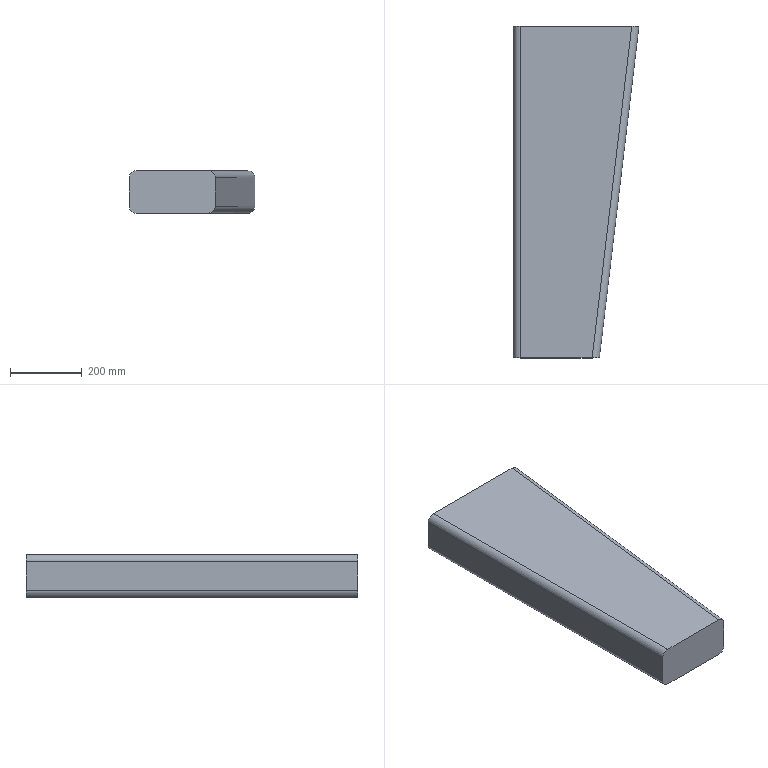Part | SolidWorks | features Extrusion 1, Fillet 1 | 1 solid | 10 faces | box 350 x 923 x 118 mm | volume 31811585 mm3 | plane 6 | cylinder 4 | commonest cylinder face diameters 40 x4
STEP:
#1=CARTESIAN_POINT('',(0.,923.,98.));
#2=VERTEX_POINT('',#1);
#3=CARTESIAN_POINT('',(0.,923.,20.));
#4=VERTEX_POINT('',#3);
#5=CARTESIAN_POINT('',(0.,923.,118.));
#6=DIRECTION('',(0.,0.,-1.));
#7=VECTOR('',#6,1000.);
#8=LINE('',#5,#7);
#9=EDGE_CURVE('',#2,#4,#8,.T.);
#10=ORIENTED_EDGE('',*,*,#9,.T.);
#11=CARTESIAN_POINT('',(0.,0.,20.));
#12=VERTEX_POINT('',#11);
#13=CARTESIAN_POINT('',(0.,923.,20.));
#14=DIRECTION('',(0.,-1.,0.));
#15=VECTOR('',#14,1000.);
#16=LINE('',#13,#15);
#17=EDGE_CURVE('',#4,#12,#16,.T.);
#18=ORIENTED_EDGE('',*,*,#17,.T.);
#19=CARTESIAN_POINT('',(0.,0.,98.));
#20=VERTEX_POINT('',#19);
#21=CARTESIAN_POINT('',(0.,0.,118.));
#22=DIRECTION('',(0.,0.,-1.));
#23=VECTOR('',#22,1000.);
#24=LINE('',#21,#23);
#25=EDGE_CURVE('',#20,#12,#24,.T.);
#26=ORIENTED_EDGE('',*,*,#25,.F.);
#27=CARTESIAN_POINT('',(0.,923.,98.));
#28=DIRECTION('',(0.,1.,0.));
#29=VECTOR('',#28,1000.);
#30=LINE('',#27,#29);
#31=EDGE_CURVE('',#20,#2,#30,.T.);
#32=ORIENTED_EDGE('',*,*,#31,.T.);
#33=EDGE_LOOP('',(#10,#18,#26,#32));
#34=FACE_OUTER_BOUND('',#33,.T.);
#35=CARTESIAN_POINT('',(0.,923.,118.));
#36=DIRECTION('',(1.,0.,0.));
#37=DIRECTION('',(0.,0.,-1.));
#38=AXIS2_PLACEMENT_3D('',#35,#36,#37);
#39=PLANE('',#38);
#40=ADVANCED_FACE('',(#34),#39,.F.);
#41=ORIENTED_EDGE('',*,*,#25,.T.);
#42=CARTESIAN_POINT('',(20.,0.,0.));
#43=VERTEX_POINT('',#42);
#44=CARTESIAN_POINT('',(20.,0.,20.));
#45=DIRECTION('',(0.,-1.,0.));
#46=DIRECTION('',(0.,0.,1.));
#47=AXIS2_PLACEMENT_3D('',#44,#45,#46);
#48=CIRCLE('',#47,20.);
#49=EDGE_CURVE('',#12,#43,#48,.T.);
#50=ORIENTED_EDGE('',*,*,#49,.T.);
#51=CARTESIAN_POINT('',(219.858,0.,0.));
#52=VERTEX_POINT('',#51);
#53=CARTESIAN_POINT('',(0.,0.,0.));
#54=DIRECTION('',(1.,0.,0.));
#55=VECTOR('',#54,1000.);
#56=LINE('',#53,#55);
#57=EDGE_CURVE('',#43,#52,#56,.T.);
#58=ORIENTED_EDGE('',*,*,#57,.T.);
#59=CARTESIAN_POINT('',(240.,0.,20.));
#60=VERTEX_POINT('',#59);
#61=CARTESIAN_POINT('',(219.858,0.,0.));
#62=CARTESIAN_POINT('',(231.657,0.,0.));
#63=CARTESIAN_POINT('',(240.,0.,8.284));
#64=CARTESIAN_POINT('',(240.,0.,20.));
#65=(BOUNDED_CURVE()B_SPLINE_CURVE(3,(#61,#62,#63,#64),.UNSPECIFIED.,.F.,.F.)B_SPLINE_CURVE_WITH_KNOTS((4,4),(4.712,6.283),.UNSPECIFIED.)CURVE()GEOMETRIC_REPRESENTATION_ITEM()RATIONAL_B_SPLINE_CURVE((1.,0.8047,0.8047,1.))REPRESENTATION_ITEM(''));
#66=EDGE_CURVE('',#52,#60,#65,.T.);
#67=ORIENTED_EDGE('',*,*,#66,.T.);
#68=CARTESIAN_POINT('',(240.,0.,98.));
#69=VERTEX_POINT('',#68);
#70=CARTESIAN_POINT('',(240.,0.,118.));
#71=DIRECTION('',(0.,0.,-1.));
#72=VECTOR('',#71,1000.);
#73=LINE('',#70,#72);
#74=EDGE_CURVE('',#69,#60,#73,.T.);
#75=ORIENTED_EDGE('',*,*,#74,.F.);
#76=CARTESIAN_POINT('',(219.858,0.,118.));
#77=VERTEX_POINT('',#76);
#78=CARTESIAN_POINT('',(240.,0.,98.));
#79=CARTESIAN_POINT('',(240.,0.,109.716));
#80=CARTESIAN_POINT('',(231.657,0.,118.));
#81=CARTESIAN_POINT('',(219.858,0.,118.));
#82=(BOUNDED_CURVE()B_SPLINE_CURVE(3,(#78,#79,#80,#81),.UNSPECIFIED.,.F.,.F.)B_SPLINE_CURVE_WITH_KNOTS((4,4),(3.142,4.712),.UNSPECIFIED.)CURVE()GEOMETRIC_REPRESENTATION_ITEM()RATIONAL_B_SPLINE_CURVE((1.,0.8047,0.8047,1.))REPRESENTATION_ITEM(''));
#83=EDGE_CURVE('',#69,#77,#82,.T.);
#84=ORIENTED_EDGE('',*,*,#83,.T.);
#85=CARTESIAN_POINT('',(20.,0.,118.));
#86=VERTEX_POINT('',#85);
#87=CARTESIAN_POINT('',(0.,0.,118.));
#88=DIRECTION('',(1.,0.,0.));
#89=VECTOR('',#88,1000.);
#90=LINE('',#87,#89);
#91=EDGE_CURVE('',#86,#77,#90,.T.);
#92=ORIENTED_EDGE('',*,*,#91,.F.);
#93=CARTESIAN_POINT('',(20.,0.,98.));
#94=DIRECTION('',(0.,-1.,0.));
#95=DIRECTION('',(0.,0.,1.));
#96=AXIS2_PLACEMENT_3D('',#93,#94,#95);
#97=CIRCLE('',#96,20.);
#98=EDGE_CURVE('',#86,#20,#97,.T.);
#99=ORIENTED_EDGE('',*,*,#98,.T.);
#100=EDGE_LOOP('',(#41,#50,#58,#67,#75,#84,#92,#99));
#101=FACE_OUTER_BOUND('',#100,.T.);
#102=CARTESIAN_POINT('',(0.,0.,118.));
#103=DIRECTION('',(0.,1.,0.));
#104=DIRECTION('',(0.,0.,1.));
#105=AXIS2_PLACEMENT_3D('',#102,#103,#104);
#106=PLANE('',#105);
#107=ADVANCED_FACE('',(#101),#106,.F.);
#108=ORIENTED_EDGE('',*,*,#74,.T.);
#109=CARTESIAN_POINT('',(350.,923.,20.));
#110=VERTEX_POINT('',#109);
#111=CARTESIAN_POINT('',(240.,0.,20.));
#112=DIRECTION('',(0.1183,0.993,0.));
#113=VECTOR('',#112,1000.);
#114=LINE('',#111,#113);
#115=EDGE_CURVE('',#60,#110,#114,.T.);
#116=ORIENTED_EDGE('',*,*,#115,.T.);
#117=CARTESIAN_POINT('',(350.,923.,98.));
#118=VERTEX_POINT('',#117);
#119=CARTESIAN_POINT('',(350.,923.,118.));
#120=DIRECTION('',(0.,0.,-1.));
#121=VECTOR('',#120,1000.);
#122=LINE('',#119,#121);
#123=EDGE_CURVE('',#118,#110,#122,.T.);
#124=ORIENTED_EDGE('',*,*,#123,.F.);
#125=CARTESIAN_POINT('',(240.,0.,98.));
#126=DIRECTION('',(-0.1183,-0.993,0.));
#127=VECTOR('',#126,1000.);
#128=LINE('',#125,#127);
#129=EDGE_CURVE('',#118,#69,#128,.T.);
#130=ORIENTED_EDGE('',*,*,#129,.T.);
#131=EDGE_LOOP('',(#108,#116,#124,#130));
#132=FACE_OUTER_BOUND('',#131,.T.);
#133=CARTESIAN_POINT('',(240.,0.,118.));
#134=DIRECTION('',(-0.993,0.1183,0.));
#135=DIRECTION('',(-0.1183,-0.993,0.));
#136=AXIS2_PLACEMENT_3D('',#133,#134,#135);
#137=PLANE('',#136);
#138=ADVANCED_FACE('',(#132),#137,.F.);
#139=CARTESIAN_POINT('',(329.858,923.,0.));
#140=VERTEX_POINT('',#139);
#141=CARTESIAN_POINT('',(20.,923.,0.));
#142=VERTEX_POINT('',#141);
#143=CARTESIAN_POINT('',(350.,923.,0.));
#144=DIRECTION('',(-1.,0.,0.));
#145=VECTOR('',#144,1000.);
#146=LINE('',#143,#145);
#147=EDGE_CURVE('',#140,#142,#146,.T.);
#148=ORIENTED_EDGE('',*,*,#147,.T.);
#149=CARTESIAN_POINT('',(20.,923.,20.));
#150=DIRECTION('',(0.,1.,0.));
#151=DIRECTION('',(1.,0.,0.));
#152=AXIS2_PLACEMENT_3D('',#149,#150,#151);
#153=CIRCLE('',#152,20.);
#154=EDGE_CURVE('',#142,#4,#153,.T.);
#155=ORIENTED_EDGE('',*,*,#154,.T.);
#156=ORIENTED_EDGE('',*,*,#9,.F.);
#157=CARTESIAN_POINT('',(20.,923.,118.));
#158=VERTEX_POINT('',#157);
#159=CARTESIAN_POINT('',(20.,923.,98.));
#160=DIRECTION('',(0.,1.,0.));
#161=DIRECTION('',(1.,0.,0.));
#162=AXIS2_PLACEMENT_3D('',#159,#160,#161);
#163=CIRCLE('',#162,20.);
#164=EDGE_CURVE('',#2,#158,#163,.T.);
#165=ORIENTED_EDGE('',*,*,#164,.T.);
#166=CARTESIAN_POINT('',(329.858,923.,118.));
#167=VERTEX_POINT('',#166);
#168=CARTESIAN_POINT('',(350.,923.,118.));
#169=DIRECTION('',(-1.,0.,0.));
#170=VECTOR('',#169,1000.);
#171=LINE('',#168,#170);
#172=EDGE_CURVE('',#167,#158,#171,.T.);
#173=ORIENTED_EDGE('',*,*,#172,.F.);
#174=CARTESIAN_POINT('',(329.858,923.,118.));
#175=CARTESIAN_POINT('',(341.657,923.,118.));
#176=CARTESIAN_POINT('',(350.,923.,109.716));
#177=CARTESIAN_POINT('',(350.,923.,98.));
#178=(BOUNDED_CURVE()B_SPLINE_CURVE(3,(#174,#175,#176,#177),.UNSPECIFIED.,.F.,.F.)B_SPLINE_CURVE_WITH_KNOTS((4,4),(1.571,3.142),.UNSPECIFIED.)CURVE()GEOMETRIC_REPRESENTATION_ITEM()RATIONAL_B_SPLINE_CURVE((1.,0.8047,0.8047,1.))REPRESENTATION_ITEM(''));
#179=EDGE_CURVE('',#167,#118,#178,.T.);
#180=ORIENTED_EDGE('',*,*,#179,.T.);
#181=ORIENTED_EDGE('',*,*,#123,.T.);
#182=CARTESIAN_POINT('',(350.,923.,20.));
#183=CARTESIAN_POINT('',(350.,923.,8.284));
#184=CARTESIAN_POINT('',(341.657,923.,0.));
#185=CARTESIAN_POINT('',(329.858,923.,0.));
#186=(BOUNDED_CURVE()B_SPLINE_CURVE(3,(#182,#183,#184,#185),.UNSPECIFIED.,.F.,.F.)B_SPLINE_CURVE_WITH_KNOTS((4,4),(0.,1.571),.UNSPECIFIED.)CURVE()GEOMETRIC_REPRESENTATION_ITEM()RATIONAL_B_SPLINE_CURVE((1.,0.8047,0.8047,1.))REPRESENTATION_ITEM(''));
#187=EDGE_CURVE('',#110,#140,#186,.T.);
#188=ORIENTED_EDGE('',*,*,#187,.T.);
#189=EDGE_LOOP('',(#148,#155,#156,#165,#173,#180,#181,#188));
#190=FACE_OUTER_BOUND('',#189,.T.);
#191=CARTESIAN_POINT('',(350.,923.,118.));
#192=DIRECTION('',(0.,-1.,0.));
#193=DIRECTION('',(1.,0.,0.));
#194=AXIS2_PLACEMENT_3D('',#191,#192,#193);
#195=PLANE('',#194);
#196=ADVANCED_FACE('',(#190),#195,.F.);
#197=ORIENTED_EDGE('',*,*,#172,.T.);
#198=CARTESIAN_POINT('',(20.,0.,118.));
#199=DIRECTION('',(0.,-1.,0.));
#200=VECTOR('',#199,1000.);
#201=LINE('',#198,#200);
#202=EDGE_CURVE('',#158,#86,#201,.T.);
#203=ORIENTED_EDGE('',*,*,#202,.T.);
#204=ORIENTED_EDGE('',*,*,#91,.T.);
#205=CARTESIAN_POINT('',(330.141,925.367,118.));
#206=DIRECTION('',(0.1183,0.993,0.));
#207=VECTOR('',#206,1000.);
#208=LINE('',#205,#207);
#209=EDGE_CURVE('',#77,#167,#208,.T.);
#210=ORIENTED_EDGE('',*,*,#209,.T.);
#211=EDGE_LOOP('',(#197,#203,#204,#210));
#212=FACE_OUTER_BOUND('',#211,.T.);
#213=CARTESIAN_POINT('',(0.,0.,118.));
#214=DIRECTION('',(0.,0.,1.));
#215=DIRECTION('',(1.,0.,0.));
#216=AXIS2_PLACEMENT_3D('',#213,#214,#215);
#217=PLANE('',#216);
#218=ADVANCED_FACE('',(#212),#217,.T.);
#219=ORIENTED_EDGE('',*,*,#57,.F.);
#220=CARTESIAN_POINT('',(20.,0.,0.));
#221=DIRECTION('',(0.,1.,0.));
#222=VECTOR('',#221,1000.);
#223=LINE('',#220,#222);
#224=EDGE_CURVE('',#43,#142,#223,.T.);
#225=ORIENTED_EDGE('',*,*,#224,.T.);
#226=ORIENTED_EDGE('',*,*,#147,.F.);
#227=CARTESIAN_POINT('',(216.78,-25.835,0.));
#228=DIRECTION('',(-0.1183,-0.993,0.));
#229=VECTOR('',#228,1000.);
#230=LINE('',#227,#229);
#231=EDGE_CURVE('',#140,#52,#230,.T.);
#232=ORIENTED_EDGE('',*,*,#231,.T.);
#233=EDGE_LOOP('',(#219,#225,#226,#232));
#234=FACE_OUTER_BOUND('',#233,.T.);
#235=CARTESIAN_POINT('',(0.,0.,0.));
#236=DIRECTION('',(0.,0.,1.));
#237=DIRECTION('',(1.,0.,0.));
#238=AXIS2_PLACEMENT_3D('',#235,#236,#237);
#239=PLANE('',#238);
#240=ADVANCED_FACE('',(#234),#239,.F.);
#241=ORIENTED_EDGE('',*,*,#154,.F.);
#242=ORIENTED_EDGE('',*,*,#224,.F.);
#243=ORIENTED_EDGE('',*,*,#49,.F.);
#244=ORIENTED_EDGE('',*,*,#17,.F.);
#245=EDGE_LOOP('',(#241,#242,#243,#244));
#246=FACE_OUTER_BOUND('',#245,.T.);
#247=CARTESIAN_POINT('',(20.,923.,20.));
#248=DIRECTION('',(0.,-1.,0.));
#249=DIRECTION('',(0.,0.,-1.));
#250=AXIS2_PLACEMENT_3D('',#247,#248,#249);
#251=CYLINDRICAL_SURFACE('',#250,20.);
#252=ADVANCED_FACE('',(#246),#251,.T.);
#253=ORIENTED_EDGE('',*,*,#164,.F.);
#254=ORIENTED_EDGE('',*,*,#31,.F.);
#255=ORIENTED_EDGE('',*,*,#98,.F.);
#256=ORIENTED_EDGE('',*,*,#202,.F.);
#257=EDGE_LOOP('',(#253,#254,#255,#256));
#258=FACE_OUTER_BOUND('',#257,.T.);
#259=CARTESIAN_POINT('',(20.,0.,98.));
#260=DIRECTION('',(0.,1.,0.));
#261=DIRECTION('',(0.,0.,1.));
#262=AXIS2_PLACEMENT_3D('',#259,#260,#261);
#263=CYLINDRICAL_SURFACE('',#262,20.);
#264=ADVANCED_FACE('',(#258),#263,.T.);
#265=ORIENTED_EDGE('',*,*,#66,.F.);
#266=ORIENTED_EDGE('',*,*,#231,.F.);
#267=ORIENTED_EDGE('',*,*,#187,.F.);
#268=ORIENTED_EDGE('',*,*,#115,.F.);
#269=EDGE_LOOP('',(#265,#266,#267,#268));
#270=FACE_OUTER_BOUND('',#269,.T.);
#271=CARTESIAN_POINT('',(220.141,2.367,20.));
#272=DIRECTION('',(0.1183,0.993,0.));
#273=DIRECTION('',(-0.993,0.1183,0.));
#274=AXIS2_PLACEMENT_3D('',#271,#272,#273);
#275=CYLINDRICAL_SURFACE('',#274,20.);
#276=ADVANCED_FACE('',(#270),#275,.T.);
#277=ORIENTED_EDGE('',*,*,#83,.F.);
#278=ORIENTED_EDGE('',*,*,#129,.F.);
#279=ORIENTED_EDGE('',*,*,#179,.F.);
#280=ORIENTED_EDGE('',*,*,#209,.F.);
#281=EDGE_LOOP('',(#277,#278,#279,#280));
#282=FACE_OUTER_BOUND('',#281,.T.);
#283=CARTESIAN_POINT('',(216.78,-25.835,98.));
#284=DIRECTION('',(-0.1183,-0.993,0.));
#285=DIRECTION('',(0.993,-0.1183,0.));
#286=AXIS2_PLACEMENT_3D('',#283,#284,#285);
#287=CYLINDRICAL_SURFACE('',#286,20.);
#288=ADVANCED_FACE('',(#282),#287,.T.);
#289=CLOSED_SHELL('',(#40,#107,#138,#196,#218,#240,#252,#264,#276,#288));
#290=MANIFOLD_SOLID_BREP('',#289);
#291=CARTESIAN_POINT('',(0.,0.,0.));
#292=DIRECTION('',(0.,0.,1.));
#293=DIRECTION('',(1.,0.,0.));
#294=AXIS2_PLACEMENT_3D('',#291,#292,#293);
#295=(LENGTH_UNIT()NAMED_UNIT(*)SI_UNIT(.MILLI.,.METRE.));
#296=UNCERTAINTY_MEASURE_WITH_UNIT(LENGTH_MEASURE(0.00001),#295,'','');
#297=(NAMED_UNIT(*)PLANE_ANGLE_UNIT()SI_UNIT($,.RADIAN.));
#298=(NAMED_UNIT(*)SI_UNIT($,.STERADIAN.)SOLID_ANGLE_UNIT());
#299=(GEOMETRIC_REPRESENTATION_CONTEXT(3)GLOBAL_UNCERTAINTY_ASSIGNED_CONTEXT((#296))GLOBAL_UNIT_ASSIGNED_CONTEXT((#295,#297,#298))REPRESENTATION_CONTEXT('',''));
#300=ADVANCED_BREP_SHAPE_REPRESENTATION('',(#290,#294),#299);